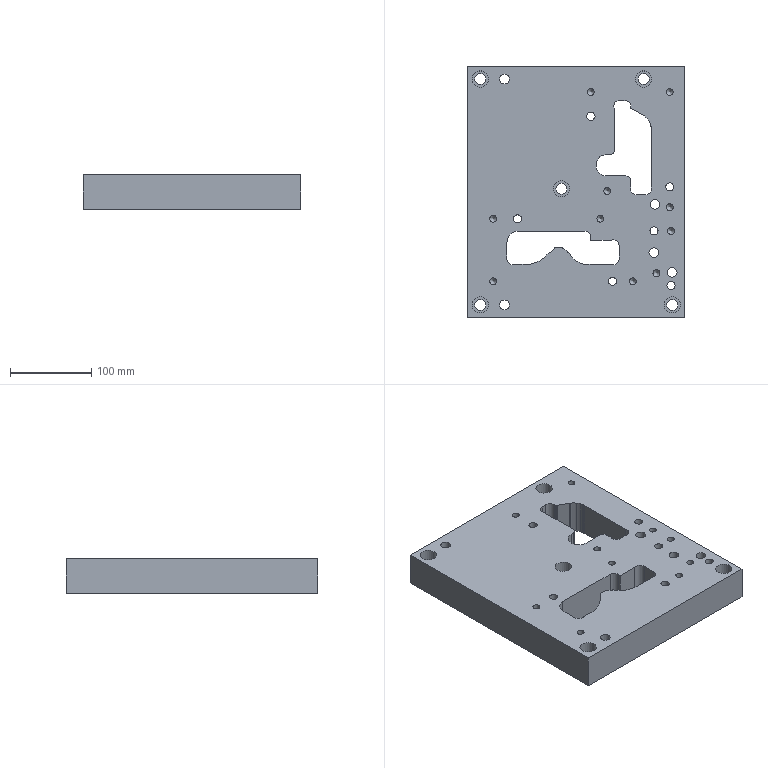Part | STEP file | lll_id4322_x_t | 1 solid | 102 faces | box 268 x 310 x 42 mm | volume 2990121 mm3 | cylinder 62 | plane 30 | cone 10 | commonest cylinder face diameters 8.506 x10 14 x8 12 x7 10 x6 13.509 x5 20.008 x5